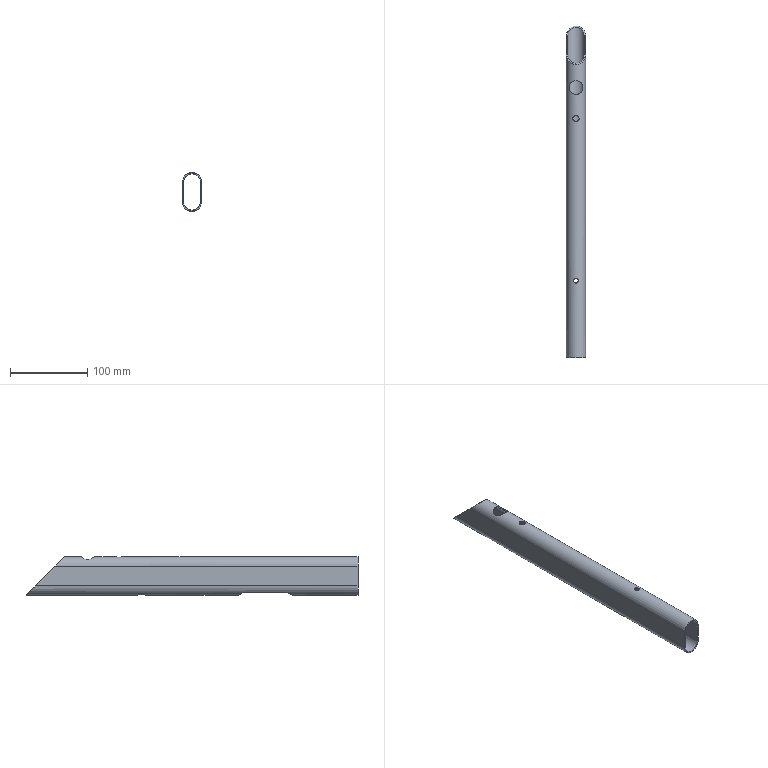Part | STEP file | 5091201R | 1 solid | 19 faces | box 25 x 430 x 50 mm | volume 72112 mm3 | cylinder 11 | plane 8 | commonest cylinder face diameters 18 x4 22 x2 25 x2 6 x1 8 x1 12 x1